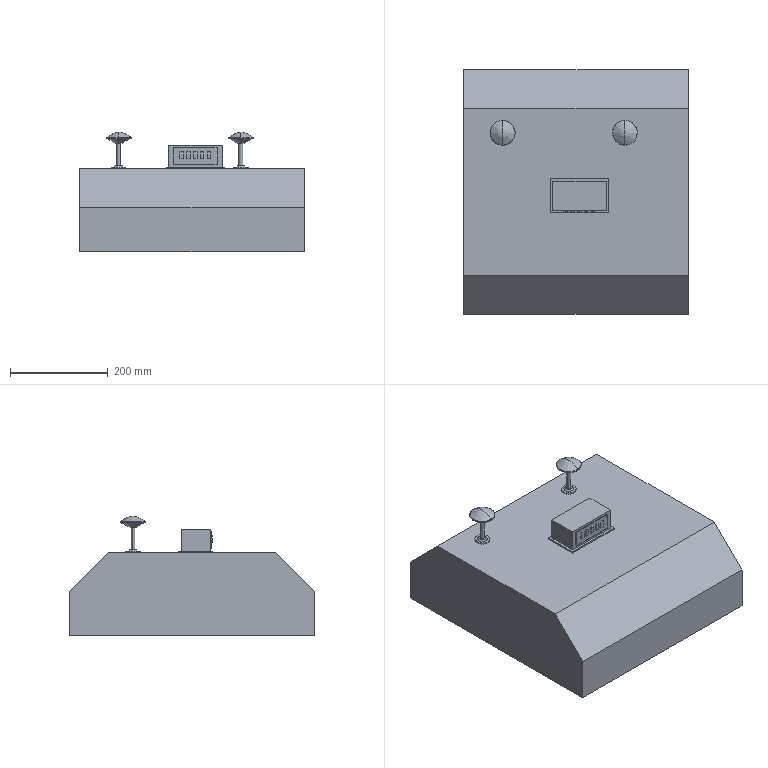Part | SolidWorks | features BaseBody 16, Chamfer 1 | 16 solids | 109 faces | box 460 x 500 x 244.744 mm | volume 2933246 mm3 | plane 81 | cylinder 16 | spline 8 | cone 4 | commonest cylinder face diameters 49.359 x6 8 x4 30 x4 51.08 x2